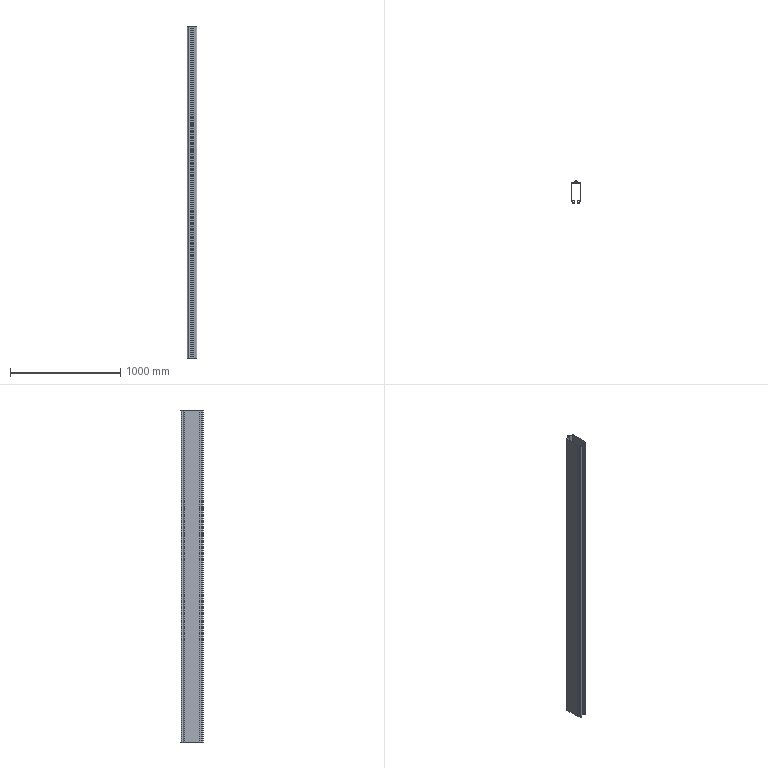Part | SolidWorks | features Extrusion 1 | 1 solid | 44 faces | box 90 x 203.757 x 3017 mm | volume 5182605 mm3 | plane 24 | cylinder 20 | commonest cylinder face diameters 14 x7 20 x7 11.964 x3 17.964 x3
STEP:
#1=CARTESIAN_POINT('',(10.,92.38,3017.));
#2=VERTEX_POINT('',#1);
#3=CARTESIAN_POINT('',(-10.,92.38,3017.));
#4=VERTEX_POINT('',#3);
#5=CARTESIAN_POINT('',(0.,92.38,3017.));
#6=DIRECTION('',(0.,0.,1.));
#7=DIRECTION('',(1.,0.,0.));
#8=AXIS2_PLACEMENT_3D('',#5,#6,#7);
#9=CIRCLE('',#8,10.);
#10=EDGE_CURVE('',#2,#4,#9,.T.);
#11=ORIENTED_EDGE('',*,*,#10,.F.);
#12=CARTESIAN_POINT('',(10.,92.38,0.));
#13=VERTEX_POINT('',#12);
#14=CARTESIAN_POINT('',(10.,92.38,3017.));
#15=DIRECTION('',(0.,0.,-1.));
#16=VECTOR('',#15,1000.);
#17=LINE('',#14,#16);
#18=EDGE_CURVE('',#2,#13,#17,.T.);
#19=ORIENTED_EDGE('',*,*,#18,.T.);
#20=CARTESIAN_POINT('',(-10.,92.38,0.));
#21=VERTEX_POINT('',#20);
#22=CARTESIAN_POINT('',(0.,92.38,0.));
#23=DIRECTION('',(0.,0.,1.));
#24=DIRECTION('',(1.,0.,0.));
#25=AXIS2_PLACEMENT_3D('',#22,#23,#24);
#26=CIRCLE('',#25,10.);
#27=EDGE_CURVE('',#13,#21,#26,.T.);
#28=ORIENTED_EDGE('',*,*,#27,.T.);
#29=CARTESIAN_POINT('',(-10.,92.38,3017.));
#30=DIRECTION('',(0.,0.,-1.));
#31=VECTOR('',#30,1000.);
#32=LINE('',#29,#31);
#33=EDGE_CURVE('',#4,#21,#32,.T.);
#34=ORIENTED_EDGE('',*,*,#33,.F.);
#35=EDGE_LOOP('',(#11,#19,#28,#34));
#36=FACE_OUTER_BOUND('',#35,.T.);
#37=CARTESIAN_POINT('',(0.,92.38,3017.));
#38=DIRECTION('',(0.,0.,-1.));
#39=DIRECTION('',(-1.,0.,0.));
#40=AXIS2_PLACEMENT_3D('',#37,#38,#39);
#41=CYLINDRICAL_SURFACE('',#40,10.);
#42=ADVANCED_FACE('',(#36),#41,.T.);
#43=CARTESIAN_POINT('',(-5.,83.72,3017.));
#44=VERTEX_POINT('',#43);
#45=CARTESIAN_POINT('',(0.,92.38,3017.));
#46=DIRECTION('',(0.,0.,1.));
#47=DIRECTION('',(1.,0.,0.));
#48=AXIS2_PLACEMENT_3D('',#45,#46,#47);
#49=CIRCLE('',#48,10.);
#50=EDGE_CURVE('',#4,#44,#49,.T.);
#51=ORIENTED_EDGE('',*,*,#50,.F.);
#52=ORIENTED_EDGE('',*,*,#33,.T.);
#53=CARTESIAN_POINT('',(-5.,83.72,0.));
#54=VERTEX_POINT('',#53);
#55=CARTESIAN_POINT('',(0.,92.38,0.));
#56=DIRECTION('',(0.,0.,1.));
#57=DIRECTION('',(1.,0.,0.));
#58=AXIS2_PLACEMENT_3D('',#55,#56,#57);
#59=CIRCLE('',#58,10.);
#60=EDGE_CURVE('',#21,#54,#59,.T.);
#61=ORIENTED_EDGE('',*,*,#60,.T.);
#62=CARTESIAN_POINT('',(-5.,83.72,3017.));
#63=DIRECTION('',(0.,0.,-1.));
#64=VECTOR('',#63,1000.);
#65=LINE('',#62,#64);
#66=EDGE_CURVE('',#44,#54,#65,.T.);
#67=ORIENTED_EDGE('',*,*,#66,.F.);
#68=EDGE_LOOP('',(#51,#52,#61,#67));
#69=FACE_OUTER_BOUND('',#68,.T.);
#70=CARTESIAN_POINT('',(0.,92.38,3017.));
#71=DIRECTION('',(0.,0.,-1.));
#72=DIRECTION('',(-1.,0.,0.));
#73=AXIS2_PLACEMENT_3D('',#70,#71,#72);
#74=CYLINDRICAL_SURFACE('',#73,10.);
#75=ADVANCED_FACE('',(#69),#74,.T.);
#76=CARTESIAN_POINT('',(7.,92.38,3017.));
#77=VERTEX_POINT('',#76);
#78=CARTESIAN_POINT('',(2.,85.672,3017.));
#79=VERTEX_POINT('',#78);
#80=CARTESIAN_POINT('',(0.,92.38,3017.));
#81=DIRECTION('',(0.,0.,-1.));
#82=DIRECTION('',(1.,0.,0.));
#83=AXIS2_PLACEMENT_3D('',#80,#81,#82);
#84=CIRCLE('',#83,7.);
#85=EDGE_CURVE('',#77,#79,#84,.T.);
#86=ORIENTED_EDGE('',*,*,#85,.F.);
#87=CARTESIAN_POINT('',(7.,92.38,0.));
#88=VERTEX_POINT('',#87);
#89=CARTESIAN_POINT('',(7.,92.38,3017.));
#90=DIRECTION('',(0.,0.,-1.));
#91=VECTOR('',#90,1000.);
#92=LINE('',#89,#91);
#93=EDGE_CURVE('',#77,#88,#92,.T.);
#94=ORIENTED_EDGE('',*,*,#93,.T.);
#95=CARTESIAN_POINT('',(2.,85.672,0.));
#96=VERTEX_POINT('',#95);
#97=CARTESIAN_POINT('',(0.,92.38,0.));
#98=DIRECTION('',(0.,0.,-1.));
#99=DIRECTION('',(1.,0.,0.));
#100=AXIS2_PLACEMENT_3D('',#97,#98,#99);
#101=CIRCLE('',#100,7.);
#102=EDGE_CURVE('',#88,#96,#101,.T.);
#103=ORIENTED_EDGE('',*,*,#102,.T.);
#104=CARTESIAN_POINT('',(2.,85.672,3017.));
#105=DIRECTION('',(0.,0.,-1.));
#106=VECTOR('',#105,1000.);
#107=LINE('',#104,#106);
#108=EDGE_CURVE('',#79,#96,#107,.T.);
#109=ORIENTED_EDGE('',*,*,#108,.F.);
#110=EDGE_LOOP('',(#86,#94,#103,#109));
#111=FACE_OUTER_BOUND('',#110,.T.);
#112=CARTESIAN_POINT('',(0.,92.38,3017.));
#113=DIRECTION('',(0.,0.,-1.));
#114=DIRECTION('',(-1.,0.,0.));
#115=AXIS2_PLACEMENT_3D('',#112,#113,#114);
#116=CYLINDRICAL_SURFACE('',#115,7.);
#117=ADVANCED_FACE('',(#111),#116,.F.);
#118=ORIENTED_EDGE('',*,*,#93,.F.);
#119=CARTESIAN_POINT('',(-7.,92.38,3017.));
#120=VERTEX_POINT('',#119);
#121=CARTESIAN_POINT('',(0.,92.38,3017.));
#122=DIRECTION('',(0.,0.,-1.));
#123=DIRECTION('',(1.,0.,0.));
#124=AXIS2_PLACEMENT_3D('',#121,#122,#123);
#125=CIRCLE('',#124,7.);
#126=EDGE_CURVE('',#120,#77,#125,.T.);
#127=ORIENTED_EDGE('',*,*,#126,.F.);
#128=CARTESIAN_POINT('',(-7.,92.38,0.));
#129=VERTEX_POINT('',#128);
#130=CARTESIAN_POINT('',(-7.,92.38,3017.));
#131=DIRECTION('',(0.,0.,-1.));
#132=VECTOR('',#131,1000.);
#133=LINE('',#130,#132);
#134=EDGE_CURVE('',#120,#129,#133,.T.);
#135=ORIENTED_EDGE('',*,*,#134,.T.);
#136=CARTESIAN_POINT('',(0.,92.38,0.));
#137=DIRECTION('',(0.,0.,-1.));
#138=DIRECTION('',(1.,0.,0.));
#139=AXIS2_PLACEMENT_3D('',#136,#137,#138);
#140=CIRCLE('',#139,7.);
#141=EDGE_CURVE('',#129,#88,#140,.T.);
#142=ORIENTED_EDGE('',*,*,#141,.T.);
#143=EDGE_LOOP('',(#118,#127,#135,#142));
#144=FACE_OUTER_BOUND('',#143,.T.);
#145=CARTESIAN_POINT('',(0.,92.38,3017.));
#146=DIRECTION('',(0.,0.,-1.));
#147=DIRECTION('',(-1.,0.,0.));
#148=AXIS2_PLACEMENT_3D('',#145,#146,#147);
#149=CYLINDRICAL_SURFACE('',#148,7.);
#150=ADVANCED_FACE('',(#144),#149,.F.);
#151=CARTESIAN_POINT('',(-32.964,-92.395,3017.));
#152=VERTEX_POINT('',#151);
#153=CARTESIAN_POINT('',(-15.,-92.395,3017.));
#154=VERTEX_POINT('',#153);
#155=CARTESIAN_POINT('',(-23.982,-92.395,3017.));
#156=DIRECTION('',(0.,0.,1.));
#157=DIRECTION('',(1.,0.,0.));
#158=AXIS2_PLACEMENT_3D('',#155,#156,#157);
#159=CIRCLE('',#158,8.982);
#160=EDGE_CURVE('',#152,#154,#159,.T.);
#161=ORIENTED_EDGE('',*,*,#160,.F.);
#162=CARTESIAN_POINT('',(-32.964,-92.395,0.));
#163=VERTEX_POINT('',#162);
#164=CARTESIAN_POINT('',(-32.964,-92.395,3017.));
#165=DIRECTION('',(0.,0.,-1.));
#166=VECTOR('',#165,1000.);
#167=LINE('',#164,#166);
#168=EDGE_CURVE('',#152,#163,#167,.T.);
#169=ORIENTED_EDGE('',*,*,#168,.T.);
#170=CARTESIAN_POINT('',(-15.,-92.395,0.));
#171=VERTEX_POINT('',#170);
#172=CARTESIAN_POINT('',(-23.982,-92.395,0.));
#173=DIRECTION('',(0.,0.,1.));
#174=DIRECTION('',(1.,0.,0.));
#175=AXIS2_PLACEMENT_3D('',#172,#173,#174);
#176=CIRCLE('',#175,8.982);
#177=EDGE_CURVE('',#163,#171,#176,.T.);
#178=ORIENTED_EDGE('',*,*,#177,.T.);
#179=CARTESIAN_POINT('',(-15.,-92.395,3017.));
#180=DIRECTION('',(0.,0.,-1.));
#181=VECTOR('',#180,1000.);
#182=LINE('',#179,#181);
#183=EDGE_CURVE('',#154,#171,#182,.T.);
#184=ORIENTED_EDGE('',*,*,#183,.F.);
#185=EDGE_LOOP('',(#161,#169,#178,#184));
#186=FACE_OUTER_BOUND('',#185,.T.);
#187=CARTESIAN_POINT('',(-23.982,-92.395,3017.));
#188=DIRECTION('',(0.,0.,-1.));
#189=DIRECTION('',(-1.,0.,0.));
#190=AXIS2_PLACEMENT_3D('',#187,#188,#189);
#191=CYLINDRICAL_SURFACE('',#190,8.982);
#192=ADVANCED_FACE('',(#186),#191,.T.);
#193=CARTESIAN_POINT('',(-29.964,-92.395,3017.));
#194=VERTEX_POINT('',#193);
#195=CARTESIAN_POINT('',(-29.504,-90.094,3017.));
#196=VERTEX_POINT('',#195);
#197=CARTESIAN_POINT('',(-23.982,-92.395,3017.));
#198=DIRECTION('',(0.,0.,-1.));
#199=DIRECTION('',(1.,0.,0.));
#200=AXIS2_PLACEMENT_3D('',#197,#198,#199);
#201=CIRCLE('',#200,5.982);
#202=EDGE_CURVE('',#194,#196,#201,.T.);
#203=ORIENTED_EDGE('',*,*,#202,.F.);
#204=CARTESIAN_POINT('',(-29.964,-92.395,0.));
#205=VERTEX_POINT('',#204);
#206=CARTESIAN_POINT('',(-29.964,-92.395,3017.));
#207=DIRECTION('',(0.,0.,-1.));
#208=VECTOR('',#207,1000.);
#209=LINE('',#206,#208);
#210=EDGE_CURVE('',#194,#205,#209,.T.);
#211=ORIENTED_EDGE('',*,*,#210,.T.);
#212=CARTESIAN_POINT('',(-29.504,-90.094,0.));
#213=VERTEX_POINT('',#212);
#214=CARTESIAN_POINT('',(-23.982,-92.395,0.));
#215=DIRECTION('',(0.,0.,-1.));
#216=DIRECTION('',(1.,0.,0.));
#217=AXIS2_PLACEMENT_3D('',#214,#215,#216);
#218=CIRCLE('',#217,5.982);
#219=EDGE_CURVE('',#205,#213,#218,.T.);
#220=ORIENTED_EDGE('',*,*,#219,.T.);
#221=CARTESIAN_POINT('',(-29.504,-90.094,3017.));
#222=DIRECTION('',(0.,0.,-1.));
#223=VECTOR('',#222,1000.);
#224=LINE('',#221,#223);
#225=EDGE_CURVE('',#196,#213,#224,.T.);
#226=ORIENTED_EDGE('',*,*,#225,.F.);
#227=EDGE_LOOP('',(#203,#211,#220,#226));
#228=FACE_OUTER_BOUND('',#227,.T.);
#229=CARTESIAN_POINT('',(-23.982,-92.395,3017.));
#230=DIRECTION('',(0.,0.,-1.));
#231=DIRECTION('',(-1.,0.,0.));
#232=AXIS2_PLACEMENT_3D('',#229,#230,#231);
#233=CYLINDRICAL_SURFACE('',#232,5.982);
#234=ADVANCED_FACE('',(#228),#233,.F.);
#235=CARTESIAN_POINT('',(-45.,-70.,0.));
#236=VERTEX_POINT('',#235);
#237=CARTESIAN_POINT('',(-35.,-80.,0.));
#238=VERTEX_POINT('',#237);
#239=CARTESIAN_POINT('',(-35.,-70.,0.));
#240=DIRECTION('',(0.,0.,1.));
#241=DIRECTION('',(1.,0.,0.));
#242=AXIS2_PLACEMENT_3D('',#239,#240,#241);
#243=CIRCLE('',#242,10.);
#244=EDGE_CURVE('',#236,#238,#243,.T.);
#245=ORIENTED_EDGE('',*,*,#244,.T.);
#246=CARTESIAN_POINT('',(-35.,-80.,3017.));
#247=VERTEX_POINT('',#246);
#248=CARTESIAN_POINT('',(-35.,-80.,3017.));
#249=DIRECTION('',(0.,0.,-1.));
#250=VECTOR('',#249,1000.);
#251=LINE('',#248,#250);
#252=EDGE_CURVE('',#247,#238,#251,.T.);
#253=ORIENTED_EDGE('',*,*,#252,.F.);
#254=CARTESIAN_POINT('',(-45.,-70.,3017.));
#255=VERTEX_POINT('',#254);
#256=CARTESIAN_POINT('',(-35.,-70.,3017.));
#257=DIRECTION('',(0.,0.,1.));
#258=DIRECTION('',(1.,0.,0.));
#259=AXIS2_PLACEMENT_3D('',#256,#257,#258);
#260=CIRCLE('',#259,10.);
#261=EDGE_CURVE('',#255,#247,#260,.T.);
#262=ORIENTED_EDGE('',*,*,#261,.F.);
#263=CARTESIAN_POINT('',(-45.,-70.,3017.));
#264=DIRECTION('',(0.,0.,-1.));
#265=VECTOR('',#264,1000.);
#266=LINE('',#263,#265);
#267=EDGE_CURVE('',#255,#236,#266,.T.);
#268=ORIENTED_EDGE('',*,*,#267,.T.);
#269=EDGE_LOOP('',(#245,#253,#262,#268));
#270=FACE_OUTER_BOUND('',#269,.T.);
#271=CARTESIAN_POINT('',(-35.,-70.,3017.));
#272=DIRECTION('',(0.,0.,-1.));
#273=DIRECTION('',(-1.,0.,0.));
#274=AXIS2_PLACEMENT_3D('',#271,#272,#273);
#275=CYLINDRICAL_SURFACE('',#274,10.);
#276=ADVANCED_FACE('',(#270),#275,.T.);
#277=CARTESIAN_POINT('',(-18.,-80.,0.));
#278=VERTEX_POINT('',#277);
#279=CARTESIAN_POINT('',(-35.,-80.,0.));
#280=DIRECTION('',(1.,0.,0.));
#281=VECTOR('',#280,1000.);
#282=LINE('',#279,#281);
#283=EDGE_CURVE('',#238,#278,#282,.T.);
#284=ORIENTED_EDGE('',*,*,#283,.T.);
#285=CARTESIAN_POINT('',(-18.,-80.,3017.));
#286=VERTEX_POINT('',#285);
#287=CARTESIAN_POINT('',(-18.,-80.,3017.));
#288=DIRECTION('',(0.,0.,-1.));
#289=VECTOR('',#288,1000.);
#290=LINE('',#287,#289);
#291=EDGE_CURVE('',#286,#278,#290,.T.);
#292=ORIENTED_EDGE('',*,*,#291,.F.);
#293=CARTESIAN_POINT('',(-35.,-80.,3017.));
#294=DIRECTION('',(1.,0.,0.));
#295=VECTOR('',#294,1000.);
#296=LINE('',#293,#295);
#297=EDGE_CURVE('',#247,#286,#296,.T.);
#298=ORIENTED_EDGE('',*,*,#297,.F.);
#299=ORIENTED_EDGE('',*,*,#252,.T.);
#300=EDGE_LOOP('',(#284,#292,#298,#299));
#301=FACE_OUTER_BOUND('',#300,.T.);
#302=CARTESIAN_POINT('',(-35.,-80.,3017.));
#303=DIRECTION('',(0.,1.,0.));
#304=DIRECTION('',(-1.,0.,0.));
#305=AXIS2_PLACEMENT_3D('',#302,#303,#304);
#306=PLANE('',#305);
#307=ADVANCED_FACE('',(#301),#306,.F.);
#308=CARTESIAN_POINT('',(-18.,-92.395,0.));
#309=VERTEX_POINT('',#308);
#310=CARTESIAN_POINT('',(-18.,-92.395,0.));
#311=DIRECTION('',(0.,-1.,0.));
#312=VECTOR('',#311,1000.);
#313=LINE('',#310,#312);
#314=EDGE_CURVE('',#278,#309,#313,.T.);
#315=ORIENTED_EDGE('',*,*,#314,.T.);
#316=CARTESIAN_POINT('',(-18.,-92.395,3017.));
#317=VERTEX_POINT('',#316);
#318=CARTESIAN_POINT('',(-18.,-92.395,3017.));
#319=DIRECTION('',(0.,0.,-1.));
#320=VECTOR('',#319,1000.);
#321=LINE('',#318,#320);
#322=EDGE_CURVE('',#317,#309,#321,.T.);
#323=ORIENTED_EDGE('',*,*,#322,.F.);
#324=CARTESIAN_POINT('',(-18.,-92.395,3017.));
#325=DIRECTION('',(0.,-1.,0.));
#326=VECTOR('',#325,1000.);
#327=LINE('',#324,#326);
#328=EDGE_CURVE('',#286,#317,#327,.T.);
#329=ORIENTED_EDGE('',*,*,#328,.F.);
#330=ORIENTED_EDGE('',*,*,#291,.T.);
#331=EDGE_LOOP('',(#315,#323,#329,#330));
#332=FACE_OUTER_BOUND('',#331,.T.);
#333=CARTESIAN_POINT('',(-18.,-92.395,3017.));
#334=DIRECTION('',(1.,0.,0.));
#335=DIRECTION('',(0.,1.,0.));
#336=AXIS2_PLACEMENT_3D('',#333,#334,#335);
#337=PLANE('',#336);
#338=ADVANCED_FACE('',(#332),#337,.F.);
#339=ORIENTED_EDGE('',*,*,#210,.F.);
#340=CARTESIAN_POINT('',(-23.982,-92.395,3017.));
#341=DIRECTION('',(0.,0.,-1.));
#342=DIRECTION('',(1.,0.,0.));
#343=AXIS2_PLACEMENT_3D('',#340,#341,#342);
#344=CIRCLE('',#343,5.982);
#345=EDGE_CURVE('',#317,#194,#344,.T.);
#346=ORIENTED_EDGE('',*,*,#345,.F.);
#347=ORIENTED_EDGE('',*,*,#322,.T.);
#348=CARTESIAN_POINT('',(-23.982,-92.395,0.));
#349=DIRECTION('',(0.,0.,-1.));
#350=DIRECTION('',(1.,0.,0.));
#351=AXIS2_PLACEMENT_3D('',#348,#349,#350);
#352=CIRCLE('',#351,5.982);
#353=EDGE_CURVE('',#309,#205,#352,.T.);
#354=ORIENTED_EDGE('',*,*,#353,.T.);
#355=EDGE_LOOP('',(#339,#346,#347,#354));
#356=FACE_OUTER_BOUND('',#355,.T.);
#357=CARTESIAN_POINT('',(-23.982,-92.395,3017.));
#358=DIRECTION('',(0.,0.,-1.));
#359=DIRECTION('',(-1.,0.,0.));
#360=AXIS2_PLACEMENT_3D('',#357,#358,#359);
#361=CYLINDRICAL_SURFACE('',#360,5.982);
#362=ADVANCED_FACE('',(#356),#361,.F.);
#363=CARTESIAN_POINT('',(-32.273,-88.94,0.));
#364=VERTEX_POINT('',#363);
#365=CARTESIAN_POINT('',(-29.504,-90.094,0.));
#366=DIRECTION('',(-0.9231,0.3846,0.));
#367=VECTOR('',#366,1000.);
#368=LINE('',#365,#367);
#369=EDGE_CURVE('',#213,#364,#368,.T.);
#370=ORIENTED_EDGE('',*,*,#369,.T.);
#371=CARTESIAN_POINT('',(-32.273,-88.94,3017.));
#372=VERTEX_POINT('',#371);
#373=CARTESIAN_POINT('',(-32.273,-88.94,3017.));
#374=DIRECTION('',(0.,0.,-1.));
#375=VECTOR('',#374,1000.);
#376=LINE('',#373,#375);
#377=EDGE_CURVE('',#372,#364,#376,.T.);
#378=ORIENTED_EDGE('',*,*,#377,.F.);
#379=CARTESIAN_POINT('',(-29.504,-90.094,3017.));
#380=DIRECTION('',(-0.9231,0.3846,0.));
#381=VECTOR('',#380,1000.);
#382=LINE('',#379,#381);
#383=EDGE_CURVE('',#196,#372,#382,.T.);
#384=ORIENTED_EDGE('',*,*,#383,.F.);
#385=ORIENTED_EDGE('',*,*,#225,.T.);
#386=EDGE_LOOP('',(#370,#378,#384,#385));
#387=FACE_OUTER_BOUND('',#386,.T.);
#388=CARTESIAN_POINT('',(-29.504,-90.094,3017.));
#389=DIRECTION('',(-0.3846,-0.9231,0.));
#390=DIRECTION('',(0.9231,-0.3846,0.));
#391=AXIS2_PLACEMENT_3D('',#388,#389,#390);
#392=PLANE('',#391);
#393=ADVANCED_FACE('',(#387),#392,.F.);
#394=ORIENTED_EDGE('',*,*,#168,.F.);
#395=CARTESIAN_POINT('',(-23.982,-92.395,3017.));
#396=DIRECTION('',(0.,0.,1.));
#397=DIRECTION('',(1.,0.,0.));
#398=AXIS2_PLACEMENT_3D('',#395,#396,#397);
#399=CIRCLE('',#398,8.982);
#400=EDGE_CURVE('',#372,#152,#399,.T.);
#401=ORIENTED_EDGE('',*,*,#400,.F.);
#402=ORIENTED_EDGE('',*,*,#377,.T.);
#403=CARTESIAN_POINT('',(-23.982,-92.395,0.));
#404=DIRECTION('',(0.,0.,1.));
#405=DIRECTION('',(1.,0.,0.));
#406=AXIS2_PLACEMENT_3D('',#403,#404,#405);
#407=CIRCLE('',#406,8.982);
#408=EDGE_CURVE('',#364,#163,#407,.T.);
#409=ORIENTED_EDGE('',*,*,#408,.T.);
#410=EDGE_LOOP('',(#394,#401,#402,#409));
#411=FACE_OUTER_BOUND('',#410,.T.);
#412=CARTESIAN_POINT('',(-23.982,-92.395,3017.));
#413=DIRECTION('',(0.,0.,-1.));
#414=DIRECTION('',(-1.,0.,0.));
#415=AXIS2_PLACEMENT_3D('',#412,#413,#414);
#416=CYLINDRICAL_SURFACE('',#415,8.982);
#417=ADVANCED_FACE('',(#411),#416,.T.);
#418=CARTESIAN_POINT('',(-15.,-77.,0.));
#419=VERTEX_POINT('',#418);
#420=CARTESIAN_POINT('',(-15.,-92.395,0.));
#421=DIRECTION('',(0.,1.,0.));
#422=VECTOR('',#421,1000.);
#423=LINE('',#420,#422);
#424=EDGE_CURVE('',#171,#419,#423,.T.);
#425=ORIENTED_EDGE('',*,*,#424,.T.);
#426=CARTESIAN_POINT('',(-15.,-77.,3017.));
#427=VERTEX_POINT('',#426);
#428=CARTESIAN_POINT('',(-15.,-77.,3017.));
#429=DIRECTION('',(0.,0.,-1.));
#430=VECTOR('',#429,1000.);
#431=LINE('',#428,#430);
#432=EDGE_CURVE('',#427,#419,#431,.T.);
#433=ORIENTED_EDGE('',*,*,#432,.F.);
#434=CARTESIAN_POINT('',(-15.,-92.395,3017.));
#435=DIRECTION('',(0.,1.,0.));
#436=VECTOR('',#435,1000.);
#437=LINE('',#434,#436);
#438=EDGE_CURVE('',#154,#427,#437,.T.);
#439=ORIENTED_EDGE('',*,*,#438,.F.);
#440=ORIENTED_EDGE('',*,*,#183,.T.);
#441=EDGE_LOOP('',(#425,#433,#439,#440));
#442=FACE_OUTER_BOUND('',#441,.T.);
#443=CARTESIAN_POINT('',(-15.,-92.395,3017.));
#444=DIRECTION('',(-1.,0.,0.));
#445=DIRECTION('',(0.,0.,1.));
#446=AXIS2_PLACEMENT_3D('',#443,#444,#445);
#447=PLANE('',#446);
#448=ADVANCED_FACE('',(#442),#447,.F.);
#449=CARTESIAN_POINT('',(-35.,-77.,0.));
#450=VERTEX_POINT('',#449);
#451=CARTESIAN_POINT('',(-35.,-77.,0.));
#452=DIRECTION('',(-1.,0.,0.));
#453=VECTOR('',#452,1000.);
#454=LINE('',#451,#453);
#455=EDGE_CURVE('',#419,#450,#454,.T.);
#456=ORIENTED_EDGE('',*,*,#455,.T.);
#457=CARTESIAN_POINT('',(-35.,-77.,3017.));
#458=VERTEX_POINT('',#457);
#459=CARTESIAN_POINT('',(-35.,-77.,3017.));
#460=DIRECTION('',(0.,0.,-1.));
#461=VECTOR('',#460,1000.);
#462=LINE('',#459,#461);
#463=EDGE_CURVE('',#458,#450,#462,.T.);
#464=ORIENTED_EDGE('',*,*,#463,.F.);
#465=CARTESIAN_POINT('',(-35.,-77.,3017.));
#466=DIRECTION('',(-1.,0.,0.));
#467=VECTOR('',#466,1000.);
#468=LINE('',#465,#467);
#469=EDGE_CURVE('',#427,#458,#468,.T.);
#470=ORIENTED_EDGE('',*,*,#469,.F.);
#471=ORIENTED_EDGE('',*,*,#432,.T.);
#472=EDGE_LOOP('',(#456,#464,#470,#471));
#473=FACE_OUTER_BOUND('',#472,.T.);
#474=CARTESIAN_POINT('',(-35.,-77.,3017.));
#475=DIRECTION('',(0.,-1.,0.));
#476=DIRECTION('',(1.,0.,0.));
#477=AXIS2_PLACEMENT_3D('',#474,#475,#476);
#478=PLANE('',#477);
#479=ADVANCED_FACE('',(#473),#478,.F.);
#480=CARTESIAN_POINT('',(-42.,-70.,0.));
#481=VERTEX_POINT('',#480);
#482=CARTESIAN_POINT('',(-35.,-70.,0.));
#483=DIRECTION('',(0.,0.,-1.));
#484=DIRECTION('',(1.,0.,0.));
#485=AXIS2_PLACEMENT_3D('',#482,#483,#484);
#486=CIRCLE('',#485,7.);
#487=EDGE_CURVE('',#450,#481,#486,.T.);
#488=ORIENTED_EDGE('',*,*,#487,.T.);
#489=CARTESIAN_POINT('',(-42.,-70.,3017.));
#490=VERTEX_POINT('',#489);
#491=CARTESIAN_POINT('',(-42.,-70.,3017.));
#492=DIRECTION('',(0.,0.,-1.));
#493=VECTOR('',#492,1000.);
#494=LINE('',#491,#493);
#495=EDGE_CURVE('',#490,#481,#494,.T.);
#496=ORIENTED_EDGE('',*,*,#495,.F.);
#497=CARTESIAN_POINT('',(-35.,-70.,3017.));
#498=DIRECTION('',(0.,0.,-1.));
#499=DIRECTION('',(1.,0.,0.));
#500=AXIS2_PLACEMENT_3D('',#497,#498,#499);
#501=CIRCLE('',#500,7.);
#502=EDGE_CURVE('',#458,#490,#501,.T.);
#503=ORIENTED_EDGE('',*,*,#502,.F.);
#504=ORIENTED_EDGE('',*,*,#463,.T.);
#505=EDGE_LOOP('',(#488,#496,#503,#504));
#506=FACE_OUTER_BOUND('',#505,.T.);
#507=CARTESIAN_POINT('',(-35.,-70.,3017.));
#508=DIRECTION('',(0.,0.,-1.));
#509=DIRECTION('',(-1.,0.,0.));
#510=AXIS2_PLACEMENT_3D('',#507,#508,#509);
#511=CYLINDRICAL_SURFACE('',#510,7.);
#512=ADVANCED_FACE('',(#506),#511,.F.);
#513=CARTESIAN_POINT('',(-42.,70.,0.));
#514=VERTEX_POINT('',#513);
#515=CARTESIAN_POINT('',(-42.,70.,0.));
#516=DIRECTION('',(0.,1.,0.));
#517=VECTOR('',#516,1000.);
#518=LINE('',#515,#517);
#519=EDGE_CURVE('',#481,#514,#518,.T.);
#520=ORIENTED_EDGE('',*,*,#519,.T.);
#521=CARTESIAN_POINT('',(-42.,70.,3017.));
#522=VERTEX_POINT('',#521);
#523=CARTESIAN_POINT('',(-42.,70.,3017.));
#524=DIRECTION('',(0.,0.,-1.));
#525=VECTOR('',#524,1000.);
#526=LINE('',#523,#525);
#527=EDGE_CURVE('',#522,#514,#526,.T.);
#528=ORIENTED_EDGE('',*,*,#527,.F.);
#529=CARTESIAN_POINT('',(-42.,70.,3017.));
#530=DIRECTION('',(0.,1.,0.));
#531=VECTOR('',#530,1000.);
#532=LINE('',#529,#531);
#533=EDGE_CURVE('',#490,#522,#532,.T.);
#534=ORIENTED_EDGE('',*,*,#533,.F.);
#535=ORIENTED_EDGE('',*,*,#495,.T.);
#536=EDGE_LOOP('',(#520,#528,#534,#535));
#537=FACE_OUTER_BOUND('',#536,.T.);
#538=CARTESIAN_POINT('',(-42.,70.,3017.));
#539=DIRECTION('',(-1.,0.,0.));
#540=DIRECTION('',(0.,0.,1.));
#541=AXIS2_PLACEMENT_3D('',#538,#539,#540);
#542=PLANE('',#541);
#543=ADVANCED_FACE('',(#537),#542,.F.);
#544=CARTESIAN_POINT('',(-35.,77.,0.));
#545=VERTEX_POINT('',#544);
#546=CARTESIAN_POINT('',(-35.,70.,0.));
#547=DIRECTION('',(0.,0.,-1.));
#548=DIRECTION('',(1.,0.,0.));
#549=AXIS2_PLACEMENT_3D('',#546,#547,#548);
#550=CIRCLE('',#549,7.);
#551=EDGE_CURVE('',#514,#545,#550,.T.);
#552=ORIENTED_EDGE('',*,*,#551,.T.);
#553=CARTESIAN_POINT('',(-35.,77.,3017.));
#554=VERTEX_POINT('',#553);
#555=CARTESIAN_POINT('',(-35.,77.,3017.));
#556=DIRECTION('',(0.,0.,-1.));
#557=VECTOR('',#556,1000.);
#558=LINE('',#555,#557);
#559=EDGE_CURVE('',#554,#545,#558,.T.);
#560=ORIENTED_EDGE('',*,*,#559,.F.);
#561=CARTESIAN_POINT('',(-35.,70.,3017.));
#562=DIRECTION('',(0.,0.,-1.));
#563=DIRECTION('',(1.,0.,0.));
#564=AXIS2_PLACEMENT_3D('',#561,#562,#563);
#565=CIRCLE('',#564,7.);
#566=EDGE_CURVE('',#522,#554,#565,.T.);
#567=ORIENTED_EDGE('',*,*,#566,.F.);
#568=ORIENTED_EDGE('',*,*,#527,.T.);
#569=EDGE_LOOP('',(#552,#560,#567,#568));
#570=FACE_OUTER_BOUND('',#569,.T.);
#571=CARTESIAN_POINT('',(-35.,70.,3017.));
#572=DIRECTION('',(0.,0.,-1.));
#573=DIRECTION('',(-1.,0.,0.));
#574=AXIS2_PLACEMENT_3D('',#571,#572,#573);
#575=CYLINDRICAL_SURFACE('',#574,7.);
#576=ADVANCED_FACE('',(#570),#575,.F.);
#577=CARTESIAN_POINT('',(-2.,77.,0.));
#578=VERTEX_POINT('',#577);
#579=CARTESIAN_POINT('',(-35.,77.,0.));
#580=DIRECTION('',(1.,0.,0.));
#581=VECTOR('',#580,1000.);
#582=LINE('',#579,#581);
#583=EDGE_CURVE('',#545,#578,#582,.T.);
#584=ORIENTED_EDGE('',*,*,#583,.T.);
#585=CARTESIAN_POINT('',(-2.,77.,3017.));
#586=VERTEX_POINT('',#585);
#587=CARTESIAN_POINT('',(-2.,77.,3017.));
#588=DIRECTION('',(0.,0.,-1.));
#589=VECTOR('',#588,1000.);
#590=LINE('',#587,#589);
#591=EDGE_CURVE('',#586,#578,#590,.T.);
#592=ORIENTED_EDGE('',*,*,#591,.F.);
#593=CARTESIAN_POINT('',(-35.,77.,3017.));
#594=DIRECTION('',(1.,0.,0.));
#595=VECTOR('',#594,1000.);
#596=LINE('',#593,#595);
#597=EDGE_CURVE('',#554,#586,#596,.T.);
#598=ORIENTED_EDGE('',*,*,#597,.F.);
#599=ORIENTED_EDGE('',*,*,#559,.T.);
#600=EDGE_LOOP('',(#584,#592,#598,#599));
#601=FACE_OUTER_BOUND('',#600,.T.);
#602=CARTESIAN_POINT('',(-35.,77.,3017.));
#603=DIRECTION('',(0.,1.,0.));
#604=DIRECTION('',(0.,0.,1.));
#605=AXIS2_PLACEMENT_3D('',#602,#603,#604);
#606=PLANE('',#605);
#607=ADVANCED_FACE('',(#601),#606,.F.);
#608=CARTESIAN_POINT('',(-2.,85.672,0.));
#609=VERTEX_POINT('',#608);
#610=CARTESIAN_POINT('',(-2.,85.672,0.));
#611=DIRECTION('',(0.,1.,0.));
#612=VECTOR('',#611,1000.);
#613=LINE('',#610,#612);
#614=EDGE_CURVE('',#578,#609,#613,.T.);
#615=ORIENTED_EDGE('',*,*,#614,.T.);
#616=CARTESIAN_POINT('',(-2.,85.672,3017.));
#617=VERTEX_POINT('',#616);
#618=CARTESIAN_POINT('',(-2.,85.672,3017.));
#619=DIRECTION('',(0.,0.,-1.));
#620=VECTOR('',#619,1000.);
#621=LINE('',#618,#620);
#622=EDGE_CURVE('',#617,#609,#621,.T.);
#623=ORIENTED_EDGE('',*,*,#622,.F.);
#624=CARTESIAN_POINT('',(-2.,85.672,3017.));
#625=DIRECTION('',(0.,1.,0.));
#626=VECTOR('',#625,1000.);
#627=LINE('',#624,#626);
#628=EDGE_CURVE('',#586,#617,#627,.T.);
#629=ORIENTED_EDGE('',*,*,#628,.F.);
#630=ORIENTED_EDGE('',*,*,#591,.T.);
#631=EDGE_LOOP('',(#615,#623,#629,#630));
#632=FACE_OUTER_BOUND('',#631,.T.);
#633=CARTESIAN_POINT('',(-2.,85.672,3017.));
#634=DIRECTION('',(-1.,0.,0.));
#635=DIRECTION('',(0.,0.,1.));
#636=AXIS2_PLACEMENT_3D('',#633,#634,#635);
#637=PLANE('',#636);
#638=ADVANCED_FACE('',(#632),#637,.F.);
#639=ORIENTED_EDGE('',*,*,#134,.F.);
#640=CARTESIAN_POINT('',(0.,92.38,3017.));
#641=DIRECTION('',(0.,0.,-1.));
#642=DIRECTION('',(1.,0.,0.));
#643=AXIS2_PLACEMENT_3D('',#640,#641,#642);
#644=CIRCLE('',#643,7.);
#645=EDGE_CURVE('',#617,#120,#644,.T.);
#646=ORIENTED_EDGE('',*,*,#645,.F.);
#647=ORIENTED_EDGE('',*,*,#622,.T.);
#648=CARTESIAN_POINT('',(0.,92.38,0.));
#649=DIRECTION('',(0.,0.,-1.));
#650=DIRECTION('',(1.,0.,0.));
#651=AXIS2_PLACEMENT_3D('',#648,#649,#650);
#652=CIRCLE('',#651,7.);
#653=EDGE_CURVE('',#609,#129,#652,.T.);
#654=ORIENTED_EDGE('',*,*,#653,.T.);
#655=EDGE_LOOP('',(#639,#646,#647,#654));
#656=FACE_OUTER_BOUND('',#655,.T.);
#657=CARTESIAN_POINT('',(0.,92.38,3017.));
#658=DIRECTION('',(0.,0.,-1.));
#659=DIRECTION('',(-1.,0.,0.));
#660=AXIS2_PLACEMENT_3D('',#657,#658,#659);
#661=CYLINDRICAL_SURFACE('',#660,7.);
#662=ADVANCED_FACE('',(#656),#661,.F.);
#663=CARTESIAN_POINT('',(2.,77.,0.));
#664=VERTEX_POINT('',#663);
#665=CARTESIAN_POINT('',(2.,85.672,0.));
#666=DIRECTION('',(0.,-1.,0.));
#667=VECTOR('',#666,1000.);
#668=LINE('',#665,#667);
#669=EDGE_CURVE('',#96,#664,#668,.T.);
#670=ORIENTED_EDGE('',*,*,#669,.T.);
#671=CARTESIAN_POINT('',(2.,77.,3017.));
#672=VERTEX_POINT('',#671);
#673=CARTESIAN_POINT('',(2.,77.,3017.));
#674=DIRECTION('',(0.,0.,-1.));
#675=VECTOR('',#674,1000.);
#676=LINE('',#673,#675);
#677=EDGE_CURVE('',#672,#664,#676,.T.);
#678=ORIENTED_EDGE('',*,*,#677,.F.);
#679=CARTESIAN_POINT('',(2.,85.672,3017.));
#680=DIRECTION('',(0.,-1.,0.));
#681=VECTOR('',#680,1000.);
#682=LINE('',#679,#681);
#683=EDGE_CURVE('',#79,#672,#682,.T.);
#684=ORIENTED_EDGE('',*,*,#683,.F.);
#685=ORIENTED_EDGE('',*,*,#108,.T.);
#686=EDGE_LOOP('',(#670,#678,#684,#685));
#687=FACE_OUTER_BOUND('',#686,.T.);
#688=CARTESIAN_POINT('',(2.,85.672,3017.));
#689=DIRECTION('',(1.,0.,0.));
#690=DIRECTION('',(0.,0.,-1.));
#691=AXIS2_PLACEMENT_3D('',#688,#689,#690);
#692=PLANE('',#691);
#693=ADVANCED_FACE('',(#687),#692,.F.);
#694=CARTESIAN_POINT('',(35.,77.,0.));
#695=VERTEX_POINT('',#694);
#696=CARTESIAN_POINT('',(2.,77.,0.));
#697=DIRECTION('',(1.,0.,0.));
#698=VECTOR('',#697,1000.);
#699=LINE('',#696,#698);
#700=EDGE_CURVE('',#664,#695,#699,.T.);
#701=ORIENTED_EDGE('',*,*,#700,.T.);
#702=CARTESIAN_POINT('',(35.,77.,3017.));
#703=VERTEX_POINT('',#702);
#704=CARTESIAN_POINT('',(35.,77.,3017.));
#705=DIRECTION('',(0.,0.,-1.));
#706=VECTOR('',#705,1000.);
#707=LINE('',#704,#706);
#708=EDGE_CURVE('',#703,#695,#707,.T.);
#709=ORIENTED_EDGE('',*,*,#708,.F.);
#710=CARTESIAN_POINT('',(2.,77.,3017.));
#711=DIRECTION('',(1.,0.,0.));
#712=VECTOR('',#711,1000.);
#713=LINE('',#710,#712);
#714=EDGE_CURVE('',#672,#703,#713,.T.);
#715=ORIENTED_EDGE('',*,*,#714,.F.);
#716=ORIENTED_EDGE('',*,*,#677,.T.);
#717=EDGE_LOOP('',(#701,#709,#715,#716));
#718=FACE_OUTER_BOUND('',#717,.T.);
#719=CARTESIAN_POINT('',(2.,77.,3017.));
#720=DIRECTION('',(0.,1.,0.));
#721=DIRECTION('',(0.,0.,1.));
#722=AXIS2_PLACEMENT_3D('',#719,#720,#721);
#723=PLANE('',#722);
#724=ADVANCED_FACE('',(#718),#723,.F.);
#725=CARTESIAN_POINT('',(42.,70.,0.));
#726=VERTEX_POINT('',#725);
#727=CARTESIAN_POINT('',(35.,70.,0.));
#728=DIRECTION('',(0.,0.,-1.));
#729=DIRECTION('',(-1.,0.,0.));
#730=AXIS2_PLACEMENT_3D('',#727,#728,#729);
#731=CIRCLE('',#730,7.);
#732=EDGE_CURVE('',#695,#726,#731,.T.);
#733=ORIENTED_EDGE('',*,*,#732,.T.);
#734=CARTESIAN_POINT('',(42.,70.,3017.));
#735=VERTEX_POINT('',#734);
#736=CARTESIAN_POINT('',(42.,70.,3017.));
#737=DIRECTION('',(0.,0.,-1.));
#738=VECTOR('',#737,1000.);
#739=LINE('',#736,#738);
#740=EDGE_CURVE('',#735,#726,#739,.T.);
#741=ORIENTED_EDGE('',*,*,#740,.F.);
#742=CARTESIAN_POINT('',(35.,70.,3017.));
#743=DIRECTION('',(0.,0.,-1.));
#744=DIRECTION('',(-1.,0.,0.));
#745=AXIS2_PLACEMENT_3D('',#742,#743,#744);
#746=CIRCLE('',#745,7.);
#747=EDGE_CURVE('',#703,#735,#746,.T.);
#748=ORIENTED_EDGE('',*,*,#747,.F.);
#749=ORIENTED_EDGE('',*,*,#708,.T.);
#750=EDGE_LOOP('',(#733,#741,#748,#749));
#751=FACE_OUTER_BOUND('',#750,.T.);
#752=CARTESIAN_POINT('',(35.,70.,3017.));
#753=DIRECTION('',(0.,0.,-1.));
#754=DIRECTION('',(-1.,0.,0.));
#755=AXIS2_PLACEMENT_3D('',#752,#753,#754);
#756=CYLINDRICAL_SURFACE('',#755,7.);
#757=ADVANCED_FACE('',(#751),#756,.F.);
#758=CARTESIAN_POINT('',(42.,-70.,0.));
#759=VERTEX_POINT('',#758);
#760=CARTESIAN_POINT('',(42.,70.,0.));
#761=DIRECTION('',(0.,-1.,0.));
#762=VECTOR('',#761,1000.);
#763=LINE('',#760,#762);
#764=EDGE_CURVE('',#726,#759,#763,.T.);
#765=ORIENTED_EDGE('',*,*,#764,.T.);
#766=CARTESIAN_POINT('',(42.,-70.,3017.));
#767=VERTEX_POINT('',#766);
#768=CARTESIAN_POINT('',(42.,-70.,3017.));
#769=DIRECTION('',(0.,0.,-1.));
#770=VECTOR('',#769,1000.);
#771=LINE('',#768,#770);
#772=EDGE_CURVE('',#767,#759,#771,.T.);
#773=ORIENTED_EDGE('',*,*,#772,.F.);
#774=CARTESIAN_POINT('',(42.,70.,3017.));
#775=DIRECTION('',(0.,-1.,0.));
#776=VECTOR('',#775,1000.);
#777=LINE('',#774,#776);
#778=EDGE_CURVE('',#735,#767,#777,.T.);
#779=ORIENTED_EDGE('',*,*,#778,.F.);
#780=ORIENTED_EDGE('',*,*,#740,.T.);
#781=EDGE_LOOP('',(#765,#773,#779,#780));
#782=FACE_OUTER_BOUND('',#781,.T.);
#783=CARTESIAN_POINT('',(42.,70.,3017.));
#784=DIRECTION('',(1.,0.,0.));
#785=DIRECTION('',(0.,1.,0.));
#786=AXIS2_PLACEMENT_3D('',#783,#784,#785);
#787=PLANE('',#786);
#788=ADVANCED_FACE('',(#782),#787,.F.);
#789=CARTESIAN_POINT('',(35.,-77.,0.));
#790=VERTEX_POINT('',#789);
#791=CARTESIAN_POINT('',(35.,-70.,0.));
#792=DIRECTION('',(0.,0.,-1.));
#793=DIRECTION('',(1.,0.,0.));
#794=AXIS2_PLACEMENT_3D('',#791,#792,#793);
#795=CIRCLE('',#794,7.);
#796=EDGE_CURVE('',#759,#790,#795,.T.);
#797=ORIENTED_EDGE('',*,*,#796,.T.);
#798=CARTESIAN_POINT('',(35.,-77.,3017.));
#799=VERTEX_POINT('',#798);
#800=CARTESIAN_POINT('',(35.,-77.,3017.));
#801=DIRECTION('',(0.,0.,-1.));
#802=VECTOR('',#801,1000.);
#803=LINE('',#800,#802);
#804=EDGE_CURVE('',#799,#790,#803,.T.);
#805=ORIENTED_EDGE('',*,*,#804,.F.);
#806=CARTESIAN_POINT('',(35.,-70.,3017.));
#807=DIRECTION('',(0.,0.,-1.));
#808=DIRECTION('',(1.,0.,0.));
#809=AXIS2_PLACEMENT_3D('',#806,#807,#808);
#810=CIRCLE('',#809,7.);
#811=EDGE_CURVE('',#767,#799,#810,.T.);
#812=ORIENTED_EDGE('',*,*,#811,.F.);
#813=ORIENTED_EDGE('',*,*,#772,.T.);
#814=EDGE_LOOP('',(#797,#805,#812,#813));
#815=FACE_OUTER_BOUND('',#814,.T.);
#816=CARTESIAN_POINT('',(35.,-70.,3017.));
#817=DIRECTION('',(0.,0.,-1.));
#818=DIRECTION('',(-1.,0.,0.));
#819=AXIS2_PLACEMENT_3D('',#816,#817,#818);
#820=CYLINDRICAL_SURFACE('',#819,7.);
#821=ADVANCED_FACE('',(#815),#820,.F.);
#822=CARTESIAN_POINT('',(15.,-77.,0.));
#823=VERTEX_POINT('',#822);
#824=CARTESIAN_POINT('',(15.,-77.,0.));
#825=DIRECTION('',(-1.,0.,0.));
#826=VECTOR('',#825,1000.);
#827=LINE('',#824,#826);
#828=EDGE_CURVE('',#790,#823,#827,.T.);
#829=ORIENTED_EDGE('',*,*,#828,.T.);
#830=CARTESIAN_POINT('',(15.,-77.,3017.));
#831=VERTEX_POINT('',#830);
#832=CARTESIAN_POINT('',(15.,-77.,3017.));
#833=DIRECTION('',(0.,0.,-1.));
#834=VECTOR('',#833,1000.);
#835=LINE('',#832,#834);
#836=EDGE_CURVE('',#831,#823,#835,.T.);
#837=ORIENTED_EDGE('',*,*,#836,.F.);
#838=CARTESIAN_POINT('',(15.,-77.,3017.));
#839=DIRECTION('',(-1.,0.,0.));
#840=VECTOR('',#839,1000.);
#841=LINE('',#838,#840);
#842=EDGE_CURVE('',#799,#831,#841,.T.);
#843=ORIENTED_EDGE('',*,*,#842,.F.);
#844=ORIENTED_EDGE('',*,*,#804,.T.);
#845=EDGE_LOOP('',(#829,#837,#843,#844));
#846=FACE_OUTER_BOUND('',#845,.T.);
#847=CARTESIAN_POINT('',(15.,-77.,3017.));
#848=DIRECTION('',(0.,-1.,0.));
#849=DIRECTION('',(1.,0.,0.));
#850=AXIS2_PLACEMENT_3D('',#847,#848,#849);
#851=PLANE('',#850);
#852=ADVANCED_FACE('',(#846),#851,.F.);
#853=CARTESIAN_POINT('',(15.,-92.395,0.));
#854=VERTEX_POINT('',#853);
#855=CARTESIAN_POINT('',(15.,-92.395,0.));
#856=DIRECTION('',(0.,-1.,0.));
#857=VECTOR('',#856,1000.);
#858=LINE('',#855,#857);
#859=EDGE_CURVE('',#823,#854,#858,.T.);
#860=ORIENTED_EDGE('',*,*,#859,.T.);
#861=CARTESIAN_POINT('',(15.,-92.395,3017.));
#862=VERTEX_POINT('',#861);
#863=CARTESIAN_POINT('',(15.,-92.395,3017.));
#864=DIRECTION('',(0.,0.,-1.));
#865=VECTOR('',#864,1000.);
#866=LINE('',#863,#865);
#867=EDGE_CURVE('',#862,#854,#866,.T.);
#868=ORIENTED_EDGE('',*,*,#867,.F.);
#869=CARTESIAN_POINT('',(15.,-92.395,3017.));
#870=DIRECTION('',(0.,-1.,0.));
#871=VECTOR('',#870,1000.);
#872=LINE('',#869,#871);
#873=EDGE_CURVE('',#831,#862,#872,.T.);
#874=ORIENTED_EDGE('',*,*,#873,.F.);
#875=ORIENTED_EDGE('',*,*,#836,.T.);
#876=EDGE_LOOP('',(#860,#868,#874,#875));
#877=FACE_OUTER_BOUND('',#876,.T.);
#878=CARTESIAN_POINT('',(15.,-92.395,3017.));
#879=DIRECTION('',(1.,0.,0.));
#880=DIRECTION('',(0.,1.,0.));
#881=AXIS2_PLACEMENT_3D('',#878,#879,#880);
#882=PLANE('',#881);
#883=ADVANCED_FACE('',(#877),#882,.F.);
#884=CARTESIAN_POINT('',(32.273,-88.94,0.));
#885=VERTEX_POINT('',#884);
#886=CARTESIAN_POINT('',(23.982,-92.395,0.));
#887=DIRECTION('',(0.,0.,1.));
#888=DIRECTION('',(-1.,0.,0.));
#889=AXIS2_PLACEMENT_3D('',#886,#887,#888);
#890=CIRCLE('',#889,8.982);
#891=EDGE_CURVE('',#854,#885,#890,.T.);
#892=ORIENTED_EDGE('',*,*,#891,.T.);
#893=CARTESIAN_POINT('',(32.273,-88.94,3017.));
#894=VERTEX_POINT('',#893);
#895=CARTESIAN_POINT('',(32.273,-88.94,3017.));
#896=DIRECTION('',(0.,0.,-1.));
#897=VECTOR('',#896,1000.);
#898=LINE('',#895,#897);
#899=EDGE_CURVE('',#894,#885,#898,.T.);
#900=ORIENTED_EDGE('',*,*,#899,.F.);
#901=CARTESIAN_POINT('',(23.982,-92.395,3017.));
#902=DIRECTION('',(0.,0.,1.));
#903=DIRECTION('',(-1.,0.,0.));
#904=AXIS2_PLACEMENT_3D('',#901,#902,#903);
#905=CIRCLE('',#904,8.982);
#906=EDGE_CURVE('',#862,#894,#905,.T.);
#907=ORIENTED_EDGE('',*,*,#906,.F.);
#908=ORIENTED_EDGE('',*,*,#867,.T.);
#909=EDGE_LOOP('',(#892,#900,#907,#908));
#910=FACE_OUTER_BOUND('',#909,.T.);
#911=CARTESIAN_POINT('',(23.982,-92.395,3017.));
#912=DIRECTION('',(0.,0.,-1.));
#913=DIRECTION('',(-1.,0.,0.));
#914=AXIS2_PLACEMENT_3D('',#911,#912,#913);
#915=CYLINDRICAL_SURFACE('',#914,8.982);
#916=ADVANCED_FACE('',(#910),#915,.T.);
#917=CARTESIAN_POINT('',(29.504,-90.094,0.));
#918=VERTEX_POINT('',#917);
#919=CARTESIAN_POINT('',(32.273,-88.94,0.));
#920=DIRECTION('',(-0.9231,-0.3846,0.));
#921=VECTOR('',#920,1000.);
#922=LINE('',#919,#921);
#923=EDGE_CURVE('',#885,#918,#922,.T.);
#924=ORIENTED_EDGE('',*,*,#923,.T.);
#925=CARTESIAN_POINT('',(29.504,-90.094,3017.));
#926=VERTEX_POINT('',#925);
#927=CARTESIAN_POINT('',(29.504,-90.094,3017.));
#928=DIRECTION('',(0.,0.,-1.));
#929=VECTOR('',#928,1000.);
#930=LINE('',#927,#929);
#931=EDGE_CURVE('',#926,#918,#930,.T.);
#932=ORIENTED_EDGE('',*,*,#931,.F.);
#933=CARTESIAN_POINT('',(32.273,-88.94,3017.));
#934=DIRECTION('',(-0.9231,-0.3846,0.));
#935=VECTOR('',#934,1000.);
#936=LINE('',#933,#935);
#937=EDGE_CURVE('',#894,#926,#936,.T.);
#938=ORIENTED_EDGE('',*,*,#937,.F.);
#939=ORIENTED_EDGE('',*,*,#899,.T.);
#940=EDGE_LOOP('',(#924,#932,#938,#939));
#941=FACE_OUTER_BOUND('',#940,.T.);
#942=CARTESIAN_POINT('',(32.273,-88.94,3017.));
#943=DIRECTION('',(0.3846,-0.9231,0.));
#944=DIRECTION('',(0.9231,0.3846,0.));
#945=AXIS2_PLACEMENT_3D('',#942,#943,#944);
#946=PLANE('',#945);
#947=ADVANCED_FACE('',(#941),#946,.F.);
#948=CARTESIAN_POINT('',(18.,-92.395,0.));
#949=VERTEX_POINT('',#948);
#950=CARTESIAN_POINT('',(23.982,-92.395,0.));
#951=DIRECTION('',(0.,0.,-1.));
#952=DIRECTION('',(-1.,0.,0.));
#953=AXIS2_PLACEMENT_3D('',#950,#951,#952);
#954=CIRCLE('',#953,5.982);
#955=EDGE_CURVE('',#918,#949,#954,.T.);
#956=ORIENTED_EDGE('',*,*,#955,.T.);
#957=CARTESIAN_POINT('',(18.,-92.395,3017.));
#958=VERTEX_POINT('',#957);
#959=CARTESIAN_POINT('',(18.,-92.395,3017.));
#960=DIRECTION('',(0.,0.,-1.));
#961=VECTOR('',#960,1000.);
#962=LINE('',#959,#961);
#963=EDGE_CURVE('',#958,#949,#962,.T.);
#964=ORIENTED_EDGE('',*,*,#963,.F.);
#965=CARTESIAN_POINT('',(23.982,-92.395,3017.));
#966=DIRECTION('',(0.,0.,-1.));
#967=DIRECTION('',(-1.,0.,0.));
#968=AXIS2_PLACEMENT_3D('',#965,#966,#967);
#969=CIRCLE('',#968,5.982);
#970=EDGE_CURVE('',#926,#958,#969,.T.);
#971=ORIENTED_EDGE('',*,*,#970,.F.);
#972=ORIENTED_EDGE('',*,*,#931,.T.);
#973=EDGE_LOOP('',(#956,#964,#971,#972));
#974=FACE_OUTER_BOUND('',#973,.T.);
#975=CARTESIAN_POINT('',(23.982,-92.395,3017.));
#976=DIRECTION('',(0.,0.,-1.));
#977=DIRECTION('',(-1.,0.,0.));
#978=AXIS2_PLACEMENT_3D('',#975,#976,#977);
#979=CYLINDRICAL_SURFACE('',#978,5.982);
#980=ADVANCED_FACE('',(#974),#979,.F.);
#981=CARTESIAN_POINT('',(18.,-80.,0.));
#982=VERTEX_POINT('',#981);
#983=CARTESIAN_POINT('',(18.,-92.395,0.));
#984=DIRECTION('',(0.,1.,0.));
#985=VECTOR('',#984,1000.);
#986=LINE('',#983,#985);
#987=EDGE_CURVE('',#949,#982,#986,.T.);
#988=ORIENTED_EDGE('',*,*,#987,.T.);
#989=CARTESIAN_POINT('',(18.,-80.,3017.));
#990=VERTEX_POINT('',#989);
#991=CARTESIAN_POINT('',(18.,-80.,3017.));
#992=DIRECTION('',(0.,0.,-1.));
#993=VECTOR('',#992,1000.);
#994=LINE('',#991,#993);
#995=EDGE_CURVE('',#990,#982,#994,.T.);
#996=ORIENTED_EDGE('',*,*,#995,.F.);
#997=CARTESIAN_POINT('',(18.,-92.395,3017.));
#998=DIRECTION('',(0.,1.,0.));
#999=VECTOR('',#998,1000.);
#1000=LINE('',#997,#999);
#1001=EDGE_CURVE('',#958,#990,#1000,.T.);
#1002=ORIENTED_EDGE('',*,*,#1001,.F.);
#1003=ORIENTED_EDGE('',*,*,#963,.T.);
#1004=EDGE_LOOP('',(#988,#996,#1002,#1003));
#1005=FACE_OUTER_BOUND('',#1004,.T.);
#1006=CARTESIAN_POINT('',(18.,-92.395,3017.));
#1007=DIRECTION('',(-1.,0.,0.));
#1008=DIRECTION('',(0.,-1.,0.));
#1009=AXIS2_PLACEMENT_3D('',#1006,#1007,#1008);
#1010=PLANE('',#1009);
#1011=ADVANCED_FACE('',(#1005),#1010,.F.);
#1012=CARTESIAN_POINT('',(35.,-80.,0.));
#1013=VERTEX_POINT('',#1012);
#1014=CARTESIAN_POINT('',(18.,-80.,0.));
#1015=DIRECTION('',(1.,0.,0.));
#1016=VECTOR('',#1015,1000.);
#1017=LINE('',#1014,#1016);
#1018=EDGE_CURVE('',#982,#1013,#1017,.T.);
#1019=ORIENTED_EDGE('',*,*,#1018,.T.);
#1020=CARTESIAN_POINT('',(35.,-80.,3017.));
#1021=VERTEX_POINT('',#1020);
#1022=CARTESIAN_POINT('',(35.,-80.,3017.));
#1023=DIRECTION('',(0.,0.,-1.));
#1024=VECTOR('',#1023,1000.);
#1025=LINE('',#1022,#1024);
#1026=EDGE_CURVE('',#1021,#1013,#1025,.T.);
#1027=ORIENTED_EDGE('',*,*,#1026,.F.);
#1028=CARTESIAN_POINT('',(18.,-80.,3017.));
#1029=DIRECTION('',(1.,0.,0.));
#1030=VECTOR('',#1029,1000.);
#1031=LINE('',#1028,#1030);
#1032=EDGE_CURVE('',#990,#1021,#1031,.T.);
#1033=ORIENTED_EDGE('',*,*,#1032,.F.);
#1034=ORIENTED_EDGE('',*,*,#995,.T.);
#1035=EDGE_LOOP('',(#1019,#1027,#1033,#1034));
#1036=FACE_OUTER_BOUND('',#1035,.T.);
#1037=CARTESIAN_POINT('',(18.,-80.,3017.));
#1038=DIRECTION('',(0.,1.,0.));
#1039=DIRECTION('',(-1.,0.,0.));
#1040=AXIS2_PLACEMENT_3D('',#1037,#1038,#1039);
#1041=PLANE('',#1040);
#1042=ADVANCED_FACE('',(#1036),#1041,.F.);
#1043=CARTESIAN_POINT('',(45.,-70.,0.));
#1044=VERTEX_POINT('',#1043);
#1045=CARTESIAN_POINT('',(35.,-70.,0.));
#1046=DIRECTION('',(0.,0.,1.));
#1047=DIRECTION('',(1.,0.,0.));
#1048=AXIS2_PLACEMENT_3D('',#1045,#1046,#1047);
#1049=CIRCLE('',#1048,10.);
#1050=EDGE_CURVE('',#1013,#1044,#1049,.T.);
#1051=ORIENTED_EDGE('',*,*,#1050,.T.);
#1052=CARTESIAN_POINT('',(45.,-70.,3017.));
#1053=VERTEX_POINT('',#1052);
#1054=CARTESIAN_POINT('',(45.,-70.,3017.));
#1055=DIRECTION('',(0.,0.,-1.));
#1056=VECTOR('',#1055,1000.);
#1057=LINE('',#1054,#1056);
#1058=EDGE_CURVE('',#1053,#1044,#1057,.T.);
#1059=ORIENTED_EDGE('',*,*,#1058,.F.);
#1060=CARTESIAN_POINT('',(35.,-70.,3017.));
#1061=DIRECTION('',(0.,0.,1.));
#1062=DIRECTION('',(1.,0.,0.));
#1063=AXIS2_PLACEMENT_3D('',#1060,#1061,#1062);
#1064=CIRCLE('',#1063,10.);
#1065=EDGE_CURVE('',#1021,#1053,#1064,.T.);
#1066=ORIENTED_EDGE('',*,*,#1065,.F.);
#1067=ORIENTED_EDGE('',*,*,#1026,.T.);
#1068=EDGE_LOOP('',(#1051,#1059,#1066,#1067));
#1069=FACE_OUTER_BOUND('',#1068,.T.);
#1070=CARTESIAN_POINT('',(35.,-70.,3017.));
#1071=DIRECTION('',(0.,0.,-1.));
#1072=DIRECTION('',(-1.,0.,0.));
#1073=AXIS2_PLACEMENT_3D('',#1070,#1071,#1072);
#1074=CYLINDRICAL_SURFACE('',#1073,10.);
#1075=ADVANCED_FACE('',(#1069),#1074,.T.);
#1076=CARTESIAN_POINT('',(45.,70.,0.));
#1077=VERTEX_POINT('',#1076);
#1078=CARTESIAN_POINT('',(45.,70.,0.));
#1079=DIRECTION('',(0.,1.,0.));
#1080=VECTOR('',#1079,1000.);
#1081=LINE('',#1078,#1080);
#1082=EDGE_CURVE('',#1044,#1077,#1081,.T.);
#1083=ORIENTED_EDGE('',*,*,#1082,.T.);
#1084=CARTESIAN_POINT('',(45.,70.,3017.));
#1085=VERTEX_POINT('',#1084);
#1086=CARTESIAN_POINT('',(45.,70.,3017.));
#1087=DIRECTION('',(0.,0.,-1.));
#1088=VECTOR('',#1087,1000.);
#1089=LINE('',#1086,#1088);
#1090=EDGE_CURVE('',#1085,#1077,#1089,.T.);
#1091=ORIENTED_EDGE('',*,*,#1090,.F.);
#1092=CARTESIAN_POINT('',(45.,70.,3017.));
#1093=DIRECTION('',(0.,1.,0.));
#1094=VECTOR('',#1093,1000.);
#1095=LINE('',#1092,#1094);
#1096=EDGE_CURVE('',#1053,#1085,#1095,.T.);
#1097=ORIENTED_EDGE('',*,*,#1096,.F.);
#1098=ORIENTED_EDGE('',*,*,#1058,.T.);
#1099=EDGE_LOOP('',(#1083,#1091,#1097,#1098));
#1100=FACE_OUTER_BOUND('',#1099,.T.);
#1101=CARTESIAN_POINT('',(45.,70.,3017.));
#1102=DIRECTION('',(-1.,0.,0.));
#1103=DIRECTION('',(0.,-1.,0.));
#1104=AXIS2_PLACEMENT_3D('',#1101,#1102,#1103);
#1105=PLANE('',#1104);
#1106=ADVANCED_FACE('',(#1100),#1105,.F.);
#1107=CARTESIAN_POINT('',(35.,80.,0.));
#1108=VERTEX_POINT('',#1107);
#1109=CARTESIAN_POINT('',(35.,70.,0.));
#1110=DIRECTION('',(0.,0.,1.));
#1111=DIRECTION('',(-1.,0.,0.));
#1112=AXIS2_PLACEMENT_3D('',#1109,#1110,#1111);
#1113=CIRCLE('',#1112,10.);
#1114=EDGE_CURVE('',#1077,#1108,#1113,.T.);
#1115=ORIENTED_EDGE('',*,*,#1114,.T.);
#1116=CARTESIAN_POINT('',(35.,80.,3017.));
#1117=VERTEX_POINT('',#1116);
#1118=CARTESIAN_POINT('',(35.,80.,3017.));
#1119=DIRECTION('',(0.,0.,-1.));
#1120=VECTOR('',#1119,1000.);
#1121=LINE('',#1118,#1120);
#1122=EDGE_CURVE('',#1117,#1108,#1121,.T.);
#1123=ORIENTED_EDGE('',*,*,#1122,.F.);
#1124=CARTESIAN_POINT('',(35.,70.,3017.));
#1125=DIRECTION('',(0.,0.,1.));
#1126=DIRECTION('',(-1.,0.,0.));
#1127=AXIS2_PLACEMENT_3D('',#1124,#1125,#1126);
#1128=CIRCLE('',#1127,10.);
#1129=EDGE_CURVE('',#1085,#1117,#1128,.T.);
#1130=ORIENTED_EDGE('',*,*,#1129,.F.);
#1131=ORIENTED_EDGE('',*,*,#1090,.T.);
#1132=EDGE_LOOP('',(#1115,#1123,#1130,#1131));
#1133=FACE_OUTER_BOUND('',#1132,.T.);
#1134=CARTESIAN_POINT('',(35.,70.,3017.));
#1135=DIRECTION('',(0.,0.,-1.));
#1136=DIRECTION('',(-1.,0.,0.));
#1137=AXIS2_PLACEMENT_3D('',#1134,#1135,#1136);
#1138=CYLINDRICAL_SURFACE('',#1137,10.);
#1139=ADVANCED_FACE('',(#1133),#1138,.T.);
#1140=CARTESIAN_POINT('',(5.,80.,0.));
#1141=VERTEX_POINT('',#1140);
#1142=CARTESIAN_POINT('',(5.,80.,0.));
#1143=DIRECTION('',(-1.,0.,0.));
#1144=VECTOR('',#1143,1000.);
#1145=LINE('',#1142,#1144);
#1146=EDGE_CURVE('',#1108,#1141,#1145,.T.);
#1147=ORIENTED_EDGE('',*,*,#1146,.T.);
#1148=CARTESIAN_POINT('',(5.,80.,3017.));
#1149=VERTEX_POINT('',#1148);
#1150=CARTESIAN_POINT('',(5.,80.,3017.));
#1151=DIRECTION('',(0.,0.,-1.));
#1152=VECTOR('',#1151,1000.);
#1153=LINE('',#1150,#1152);
#1154=EDGE_CURVE('',#1149,#1141,#1153,.T.);
#1155=ORIENTED_EDGE('',*,*,#1154,.F.);
#1156=CARTESIAN_POINT('',(5.,80.,3017.));
#1157=DIRECTION('',(-1.,0.,0.));
#1158=VECTOR('',#1157,1000.);
#1159=LINE('',#1156,#1158);
#1160=EDGE_CURVE('',#1117,#1149,#1159,.T.);
#1161=ORIENTED_EDGE('',*,*,#1160,.F.);
#1162=ORIENTED_EDGE('',*,*,#1122,.T.);
#1163=EDGE_LOOP('',(#1147,#1155,#1161,#1162));
#1164=FACE_OUTER_BOUND('',#1163,.T.);
#1165=CARTESIAN_POINT('',(5.,80.,3017.));
#1166=DIRECTION('',(0.,-1.,0.));
#1167=DIRECTION('',(0.,0.,-1.));
#1168=AXIS2_PLACEMENT_3D('',#1165,#1166,#1167);
#1169=PLANE('',#1168);
#1170=ADVANCED_FACE('',(#1164),#1169,.F.);
#1171=CARTESIAN_POINT('',(5.,83.72,0.));
#1172=VERTEX_POINT('',#1171);
#1173=CARTESIAN_POINT('',(5.,83.72,0.));
#1174=DIRECTION('',(0.,1.,0.));
#1175=VECTOR('',#1174,1000.);
#1176=LINE('',#1173,#1175);
#1177=EDGE_CURVE('',#1141,#1172,#1176,.T.);
#1178=ORIENTED_EDGE('',*,*,#1177,.T.);
#1179=CARTESIAN_POINT('',(5.,83.72,3017.));
#1180=VERTEX_POINT('',#1179);
#1181=CARTESIAN_POINT('',(5.,83.72,3017.));
#1182=DIRECTION('',(0.,0.,-1.));
#1183=VECTOR('',#1182,1000.);
#1184=LINE('',#1181,#1183);
#1185=EDGE_CURVE('',#1180,#1172,#1184,.T.);
#1186=ORIENTED_EDGE('',*,*,#1185,.F.);
#1187=CARTESIAN_POINT('',(5.,83.72,3017.));
#1188=DIRECTION('',(0.,1.,0.));
#1189=VECTOR('',#1188,1000.);
#1190=LINE('',#1187,#1189);
#1191=EDGE_CURVE('',#1149,#1180,#1190,.T.);
#1192=ORIENTED_EDGE('',*,*,#1191,.F.);
#1193=ORIENTED_EDGE('',*,*,#1154,.T.);
#1194=EDGE_LOOP('',(#1178,#1186,#1192,#1193));
#1195=FACE_OUTER_BOUND('',#1194,.T.);
#1196=CARTESIAN_POINT('',(5.,83.72,3017.));
#1197=DIRECTION('',(-1.,0.,0.));
#1198=DIRECTION('',(0.,-1.,0.));
#1199=AXIS2_PLACEMENT_3D('',#1196,#1197,#1198);
#1200=PLANE('',#1199);
#1201=ADVANCED_FACE('',(#1195),#1200,.F.);
#1202=ORIENTED_EDGE('',*,*,#18,.F.);
#1203=CARTESIAN_POINT('',(0.,92.38,3017.));
#1204=DIRECTION('',(0.,0.,1.));
#1205=DIRECTION('',(1.,0.,0.));
#1206=AXIS2_PLACEMENT_3D('',#1203,#1204,#1205);
#1207=CIRCLE('',#1206,10.);
#1208=EDGE_CURVE('',#1180,#2,#1207,.T.);
#1209=ORIENTED_EDGE('',*,*,#1208,.F.);
#1210=ORIENTED_EDGE('',*,*,#1185,.T.);
#1211=CARTESIAN_POINT('',(0.,92.38,0.));
#1212=DIRECTION('',(0.,0.,1.));
#1213=DIRECTION('',(1.,0.,0.));
#1214=AXIS2_PLACEMENT_3D('',#1211,#1212,#1213);
#1215=CIRCLE('',#1214,10.);
#1216=EDGE_CURVE('',#1172,#13,#1215,.T.);
#1217=ORIENTED_EDGE('',*,*,#1216,.T.);
#1218=EDGE_LOOP('',(#1202,#1209,#1210,#1217));
#1219=FACE_OUTER_BOUND('',#1218,.T.);
#1220=CARTESIAN_POINT('',(0.,92.38,3017.));
#1221=DIRECTION('',(0.,0.,-1.));
#1222=DIRECTION('',(-1.,0.,0.));
#1223=AXIS2_PLACEMENT_3D('',#1220,#1221,#1222);
#1224=CYLINDRICAL_SURFACE('',#1223,10.);
#1225=ADVANCED_FACE('',(#1219),#1224,.T.);
#1226=CARTESIAN_POINT('',(-5.,80.,0.));
#1227=VERTEX_POINT('',#1226);
#1228=CARTESIAN_POINT('',(-5.,83.72,0.));
#1229=DIRECTION('',(0.,-1.,0.));
#1230=VECTOR('',#1229,1000.);
#1231=LINE('',#1228,#1230);
#1232=EDGE_CURVE('',#54,#1227,#1231,.T.);
#1233=ORIENTED_EDGE('',*,*,#1232,.T.);
#1234=CARTESIAN_POINT('',(-5.,80.,3017.));
#1235=VERTEX_POINT('',#1234);
#1236=CARTESIAN_POINT('',(-5.,80.,3017.));
#1237=DIRECTION('',(0.,0.,-1.));
#1238=VECTOR('',#1237,1000.);
#1239=LINE('',#1236,#1238);
#1240=EDGE_CURVE('',#1235,#1227,#1239,.T.);
#1241=ORIENTED_EDGE('',*,*,#1240,.F.);
#1242=CARTESIAN_POINT('',(-5.,83.72,3017.));
#1243=DIRECTION('',(0.,-1.,0.));
#1244=VECTOR('',#1243,1000.);
#1245=LINE('',#1242,#1244);
#1246=EDGE_CURVE('',#44,#1235,#1245,.T.);
#1247=ORIENTED_EDGE('',*,*,#1246,.F.);
#1248=ORIENTED_EDGE('',*,*,#66,.T.);
#1249=EDGE_LOOP('',(#1233,#1241,#1247,#1248));
#1250=FACE_OUTER_BOUND('',#1249,.T.);
#1251=CARTESIAN_POINT('',(-5.,83.72,3017.));
#1252=DIRECTION('',(1.,0.,0.));
#1253=DIRECTION('',(0.,1.,0.));
#1254=AXIS2_PLACEMENT_3D('',#1251,#1252,#1253);
#1255=PLANE('',#1254);
#1256=ADVANCED_FACE('',(#1250),#1255,.F.);
#1257=CARTESIAN_POINT('',(-35.,80.,0.));
#1258=VERTEX_POINT('',#1257);
#1259=CARTESIAN_POINT('',(-35.,80.,0.));
#1260=DIRECTION('',(-1.,0.,0.));
#1261=VECTOR('',#1260,1000.);
#1262=LINE('',#1259,#1261);
#1263=EDGE_CURVE('',#1227,#1258,#1262,.T.);
#1264=ORIENTED_EDGE('',*,*,#1263,.T.);
#1265=CARTESIAN_POINT('',(-35.,80.,3017.));
#1266=VERTEX_POINT('',#1265);
#1267=CARTESIAN_POINT('',(-35.,80.,3017.));
#1268=DIRECTION('',(0.,0.,-1.));
#1269=VECTOR('',#1268,1000.);
#1270=LINE('',#1267,#1269);
#1271=EDGE_CURVE('',#1266,#1258,#1270,.T.);
#1272=ORIENTED_EDGE('',*,*,#1271,.F.);
#1273=CARTESIAN_POINT('',(-35.,80.,3017.));
#1274=DIRECTION('',(-1.,0.,0.));
#1275=VECTOR('',#1274,1000.);
#1276=LINE('',#1273,#1275);
#1277=EDGE_CURVE('',#1235,#1266,#1276,.T.);
#1278=ORIENTED_EDGE('',*,*,#1277,.F.);
#1279=ORIENTED_EDGE('',*,*,#1240,.T.);
#1280=EDGE_LOOP('',(#1264,#1272,#1278,#1279));
#1281=FACE_OUTER_BOUND('',#1280,.T.);
#1282=CARTESIAN_POINT('',(-35.,80.,3017.));
#1283=DIRECTION('',(0.,-1.,0.));
#1284=DIRECTION('',(0.,0.,-1.));
#1285=AXIS2_PLACEMENT_3D('',#1282,#1283,#1284);
#1286=PLANE('',#1285);
#1287=ADVANCED_FACE('',(#1281),#1286,.F.);
#1288=CARTESIAN_POINT('',(-45.,70.,0.));
#1289=VERTEX_POINT('',#1288);
#1290=CARTESIAN_POINT('',(-35.,70.,0.));
#1291=DIRECTION('',(0.,0.,1.));
#1292=DIRECTION('',(1.,0.,0.));
#1293=AXIS2_PLACEMENT_3D('',#1290,#1291,#1292);
#1294=CIRCLE('',#1293,10.);
#1295=EDGE_CURVE('',#1258,#1289,#1294,.T.);
#1296=ORIENTED_EDGE('',*,*,#1295,.T.);
#1297=CARTESIAN_POINT('',(-45.,70.,3017.));
#1298=VERTEX_POINT('',#1297);
#1299=CARTESIAN_POINT('',(-45.,70.,3017.));
#1300=DIRECTION('',(0.,0.,-1.));
#1301=VECTOR('',#1300,1000.);
#1302=LINE('',#1299,#1301);
#1303=EDGE_CURVE('',#1298,#1289,#1302,.T.);
#1304=ORIENTED_EDGE('',*,*,#1303,.F.);
#1305=CARTESIAN_POINT('',(-35.,70.,3017.));
#1306=DIRECTION('',(0.,0.,1.));
#1307=DIRECTION('',(1.,0.,0.));
#1308=AXIS2_PLACEMENT_3D('',#1305,#1306,#1307);
#1309=CIRCLE('',#1308,10.);
#1310=EDGE_CURVE('',#1266,#1298,#1309,.T.);
#1311=ORIENTED_EDGE('',*,*,#1310,.F.);
#1312=ORIENTED_EDGE('',*,*,#1271,.T.);
#1313=EDGE_LOOP('',(#1296,#1304,#1311,#1312));
#1314=FACE_OUTER_BOUND('',#1313,.T.);
#1315=CARTESIAN_POINT('',(-35.,70.,3017.));
#1316=DIRECTION('',(0.,0.,-1.));
#1317=DIRECTION('',(-1.,0.,0.));
#1318=AXIS2_PLACEMENT_3D('',#1315,#1316,#1317);
#1319=CYLINDRICAL_SURFACE('',#1318,10.);
#1320=ADVANCED_FACE('',(#1314),#1319,.T.);
#1321=CARTESIAN_POINT('',(-45.,70.,0.));
#1322=DIRECTION('',(0.,-1.,0.));
#1323=VECTOR('',#1322,1000.);
#1324=LINE('',#1321,#1323);
#1325=EDGE_CURVE('',#1289,#236,#1324,.T.);
#1326=ORIENTED_EDGE('',*,*,#1325,.T.);
#1327=ORIENTED_EDGE('',*,*,#267,.F.);
#1328=CARTESIAN_POINT('',(-45.,70.,3017.));
#1329=DIRECTION('',(0.,-1.,0.));
#1330=VECTOR('',#1329,1000.);
#1331=LINE('',#1328,#1330);
#1332=EDGE_CURVE('',#1298,#255,#1331,.T.);
#1333=ORIENTED_EDGE('',*,*,#1332,.F.);
#1334=ORIENTED_EDGE('',*,*,#1303,.T.);
#1335=EDGE_LOOP('',(#1326,#1327,#1333,#1334));
#1336=FACE_OUTER_BOUND('',#1335,.T.);
#1337=CARTESIAN_POINT('',(-45.,70.,3017.));
#1338=DIRECTION('',(1.,0.,0.));
#1339=DIRECTION('',(0.,1.,0.));
#1340=AXIS2_PLACEMENT_3D('',#1337,#1338,#1339);
#1341=PLANE('',#1340);
#1342=ADVANCED_FACE('',(#1336),#1341,.F.);
#1343=ORIENTED_EDGE('',*,*,#261,.T.);
#1344=ORIENTED_EDGE('',*,*,#297,.T.);
#1345=ORIENTED_EDGE('',*,*,#328,.T.);
#1346=ORIENTED_EDGE('',*,*,#345,.T.);
#1347=ORIENTED_EDGE('',*,*,#202,.T.);
#1348=ORIENTED_EDGE('',*,*,#383,.T.);
#1349=ORIENTED_EDGE('',*,*,#400,.T.);
#1350=ORIENTED_EDGE('',*,*,#160,.T.);
#1351=ORIENTED_EDGE('',*,*,#438,.T.);
#1352=ORIENTED_EDGE('',*,*,#469,.T.);
#1353=ORIENTED_EDGE('',*,*,#502,.T.);
#1354=ORIENTED_EDGE('',*,*,#533,.T.);
#1355=ORIENTED_EDGE('',*,*,#566,.T.);
#1356=ORIENTED_EDGE('',*,*,#597,.T.);
#1357=ORIENTED_EDGE('',*,*,#628,.T.);
#1358=ORIENTED_EDGE('',*,*,#645,.T.);
#1359=ORIENTED_EDGE('',*,*,#126,.T.);
#1360=ORIENTED_EDGE('',*,*,#85,.T.);
#1361=ORIENTED_EDGE('',*,*,#683,.T.);
#1362=ORIENTED_EDGE('',*,*,#714,.T.);
#1363=ORIENTED_EDGE('',*,*,#747,.T.);
#1364=ORIENTED_EDGE('',*,*,#778,.T.);
#1365=ORIENTED_EDGE('',*,*,#811,.T.);
#1366=ORIENTED_EDGE('',*,*,#842,.T.);
#1367=ORIENTED_EDGE('',*,*,#873,.T.);
#1368=ORIENTED_EDGE('',*,*,#906,.T.);
#1369=ORIENTED_EDGE('',*,*,#937,.T.);
#1370=ORIENTED_EDGE('',*,*,#970,.T.);
#1371=ORIENTED_EDGE('',*,*,#1001,.T.);
#1372=ORIENTED_EDGE('',*,*,#1032,.T.);
#1373=ORIENTED_EDGE('',*,*,#1065,.T.);
#1374=ORIENTED_EDGE('',*,*,#1096,.T.);
#1375=ORIENTED_EDGE('',*,*,#1129,.T.);
#1376=ORIENTED_EDGE('',*,*,#1160,.T.);
#1377=ORIENTED_EDGE('',*,*,#1191,.T.);
#1378=ORIENTED_EDGE('',*,*,#1208,.T.);
#1379=ORIENTED_EDGE('',*,*,#10,.T.);
#1380=ORIENTED_EDGE('',*,*,#50,.T.);
#1381=ORIENTED_EDGE('',*,*,#1246,.T.);
#1382=ORIENTED_EDGE('',*,*,#1277,.T.);
#1383=ORIENTED_EDGE('',*,*,#1310,.T.);
#1384=ORIENTED_EDGE('',*,*,#1332,.T.);
#1385=EDGE_LOOP('',(#1343,#1344,#1345,#1346,#1347,#1348,#1349,#1350,#1351,#1352,#1353,#1354,#1355,#1356,#1357,#1358,#1359,#1360,#1361,#1362,#1363,#1364,#1365,#1366,#1367,#1368,#1369,#1370,#1371,#1372,#1373,#1374,#1375,#1376,#1377,#1378,#1379,#1380,#1381,#1382,#1383,#1384));
#1386=FACE_OUTER_BOUND('',#1385,.T.);
#1387=CARTESIAN_POINT('',(-35.,-70.,3017.));
#1388=DIRECTION('',(0.,0.,1.));
#1389=DIRECTION('',(1.,0.,0.));
#1390=AXIS2_PLACEMENT_3D('',#1387,#1388,#1389);
#1391=PLANE('',#1390);
#1392=ADVANCED_FACE('',(#1386),#1391,.T.);
#1393=ORIENTED_EDGE('',*,*,#244,.F.);
#1394=ORIENTED_EDGE('',*,*,#1325,.F.);
#1395=ORIENTED_EDGE('',*,*,#1295,.F.);
#1396=ORIENTED_EDGE('',*,*,#1263,.F.);
#1397=ORIENTED_EDGE('',*,*,#1232,.F.);
#1398=ORIENTED_EDGE('',*,*,#60,.F.);
#1399=ORIENTED_EDGE('',*,*,#27,.F.);
#1400=ORIENTED_EDGE('',*,*,#1216,.F.);
#1401=ORIENTED_EDGE('',*,*,#1177,.F.);
#1402=ORIENTED_EDGE('',*,*,#1146,.F.);
#1403=ORIENTED_EDGE('',*,*,#1114,.F.);
#1404=ORIENTED_EDGE('',*,*,#1082,.F.);
#1405=ORIENTED_EDGE('',*,*,#1050,.F.);
#1406=ORIENTED_EDGE('',*,*,#1018,.F.);
#1407=ORIENTED_EDGE('',*,*,#987,.F.);
#1408=ORIENTED_EDGE('',*,*,#955,.F.);
#1409=ORIENTED_EDGE('',*,*,#923,.F.);
#1410=ORIENTED_EDGE('',*,*,#891,.F.);
#1411=ORIENTED_EDGE('',*,*,#859,.F.);
#1412=ORIENTED_EDGE('',*,*,#828,.F.);
#1413=ORIENTED_EDGE('',*,*,#796,.F.);
#1414=ORIENTED_EDGE('',*,*,#764,.F.);
#1415=ORIENTED_EDGE('',*,*,#732,.F.);
#1416=ORIENTED_EDGE('',*,*,#700,.F.);
#1417=ORIENTED_EDGE('',*,*,#669,.F.);
#1418=ORIENTED_EDGE('',*,*,#102,.F.);
#1419=ORIENTED_EDGE('',*,*,#141,.F.);
#1420=ORIENTED_EDGE('',*,*,#653,.F.);
#1421=ORIENTED_EDGE('',*,*,#614,.F.);
#1422=ORIENTED_EDGE('',*,*,#583,.F.);
#1423=ORIENTED_EDGE('',*,*,#551,.F.);
#1424=ORIENTED_EDGE('',*,*,#519,.F.);
#1425=ORIENTED_EDGE('',*,*,#487,.F.);
#1426=ORIENTED_EDGE('',*,*,#455,.F.);
#1427=ORIENTED_EDGE('',*,*,#424,.F.);
#1428=ORIENTED_EDGE('',*,*,#177,.F.);
#1429=ORIENTED_EDGE('',*,*,#408,.F.);
#1430=ORIENTED_EDGE('',*,*,#369,.F.);
#1431=ORIENTED_EDGE('',*,*,#219,.F.);
#1432=ORIENTED_EDGE('',*,*,#353,.F.);
#1433=ORIENTED_EDGE('',*,*,#314,.F.);
#1434=ORIENTED_EDGE('',*,*,#283,.F.);
#1435=EDGE_LOOP('',(#1393,#1394,#1395,#1396,#1397,#1398,#1399,#1400,#1401,#1402,#1403,#1404,#1405,#1406,#1407,#1408,#1409,#1410,#1411,#1412,#1413,#1414,#1415,#1416,#1417,#1418,#1419,#1420,#1421,#1422,#1423,#1424,#1425,#1426,#1427,#1428,#1429,#1430,#1431,#1432,#1433,#1434));
#1436=FACE_OUTER_BOUND('',#1435,.T.);
#1437=CARTESIAN_POINT('',(-35.,-70.,0.));
#1438=DIRECTION('',(0.,0.,1.));
#1439=DIRECTION('',(1.,0.,0.));
#1440=AXIS2_PLACEMENT_3D('',#1437,#1438,#1439);
#1441=PLANE('',#1440);
#1442=ADVANCED_FACE('',(#1436),#1441,.F.);
#1443=CLOSED_SHELL('',(#42,#75,#117,#150,#192,#234,#276,#307,#338,#362,#393,#417,#448,#479,#512,#543,#576,#607,#638,#662,#693,#724,#757,#788,#821,#852,#883,#916,#947,#980,#1011,#1042,#1075,#1106,#1139,#1170,#1201,#1225,#1256,#1287,#1320,#1342,#1392,#1442));
#1444=MANIFOLD_SOLID_BREP('',#1443);
#1445=CARTESIAN_POINT('',(0.,0.,0.));
#1446=DIRECTION('',(0.,0.,1.));
#1447=DIRECTION('',(1.,0.,0.));
#1448=AXIS2_PLACEMENT_3D('',#1445,#1446,#1447);
#1449=(LENGTH_UNIT()NAMED_UNIT(*)SI_UNIT(.MILLI.,.METRE.));
#1450=UNCERTAINTY_MEASURE_WITH_UNIT(LENGTH_MEASURE(0.00001),#1449,'','');
#1451=(NAMED_UNIT(*)PLANE_ANGLE_UNIT()SI_UNIT($,.RADIAN.));
#1452=(NAMED_UNIT(*)SI_UNIT($,.STERADIAN.)SOLID_ANGLE_UNIT());
#1453=(GEOMETRIC_REPRESENTATION_CONTEXT(3)GLOBAL_UNCERTAINTY_ASSIGNED_CONTEXT((#1450))GLOBAL_UNIT_ASSIGNED_CONTEXT((#1449,#1451,#1452))REPRESENTATION_CONTEXT('',''));
#1454=ADVANCED_BREP_SHAPE_REPRESENTATION('',(#1444,#1448),#1453);